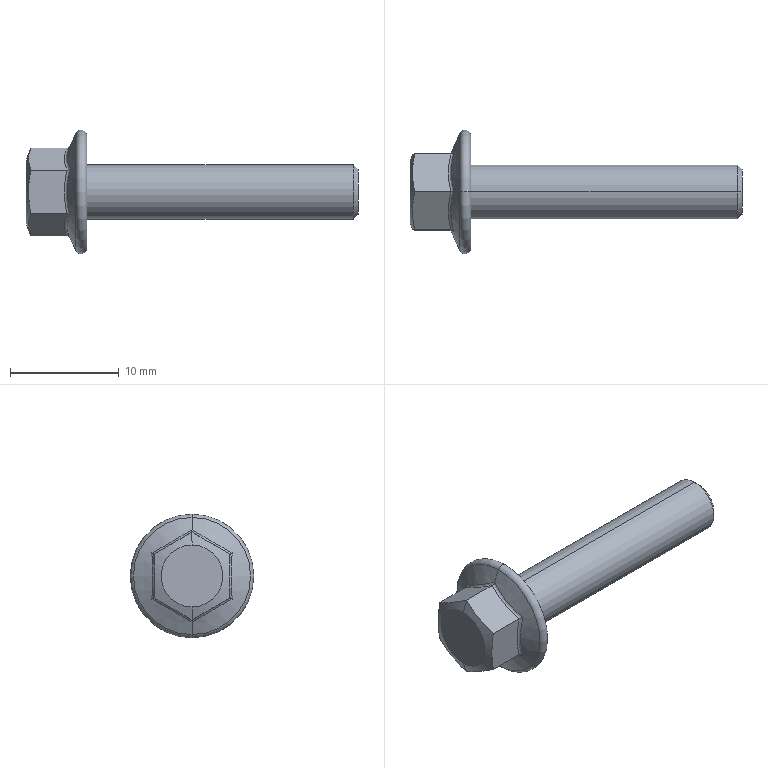Part | STEP file | hexagon flange bolts--small series gbV1.201001_GB_FASTENER_BOLT_HFBSS M5X25-N | 1 solid | 25 faces | box 30.6 x 11.4 x 11.4 mm | volume 799.257 mm3 | plane 9 | cone 6 | spline 6 | torus 2 | cylinder 2 | commonest cylinder face diameters 5 x2